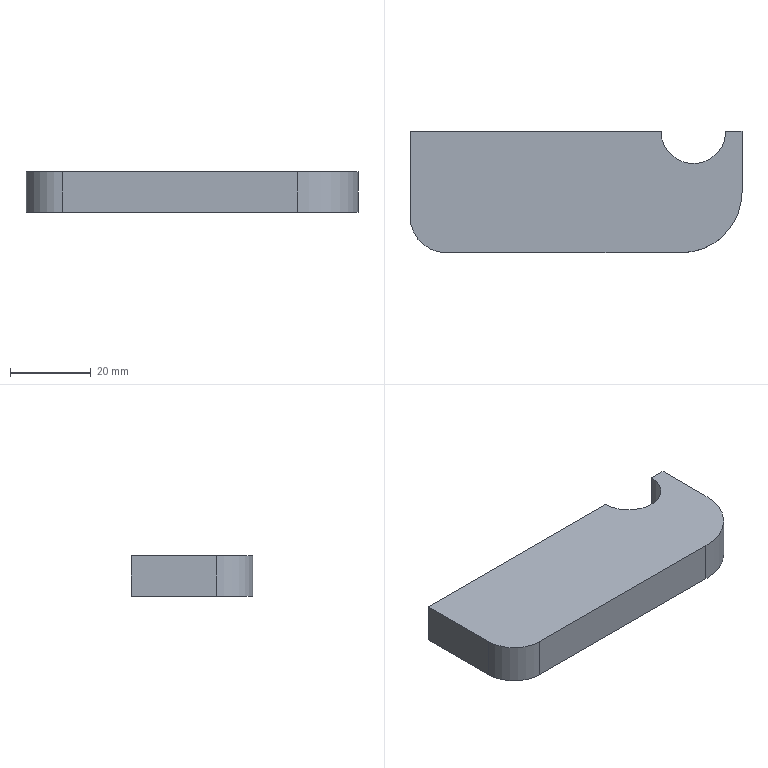Part | STEP file | Part 5_Default<As machined> | 1 solid | 10 faces | box 82 x 30 x 10 mm | volume 22938 mm3 | plane 7 | cylinder 3 | commonest cylinder face diameters 16 x1 18 x1 30 x1
STEP:
#1=CARTESIAN_POINT('',(0.,0.,0.));
#2=DIRECTION('',(0.,0.,1.));
#3=DIRECTION('',(1.,0.,0.));
#4=AXIS2_PLACEMENT_3D('',#1,#2,#3);
#5=CARTESIAN_POINT('',(9.,0.,5.));
#6=VERTEX_POINT('',#5);
#7=CARTESIAN_POINT('',(67.,0.,5.));
#8=VERTEX_POINT('',#7);
#9=CARTESIAN_POINT('',(67.,0.,5.));
#10=DIRECTION('',(1.,0.,0.));
#11=VECTOR('',#10,1.);
#12=LINE('',#9,#11);
#13=CARTESIAN_POINT('',(67.,0.,5.));
#14=DIRECTION('',(0.,1.,0.));
#15=DIRECTION('',(-1.,0.,0.));
#16=AXIS2_PLACEMENT_3D('',#13,#14,#15);
#17=PLANE('',#16);
#18=CARTESIAN_POINT('',(0.,0.));
#19=DIRECTION('',(-1.,0.));
#20=VECTOR('',#19,1.);
#21=LINE('',#18,#20);
#22=(GEOMETRIC_REPRESENTATION_CONTEXT(2)PARAMETRIC_REPRESENTATION_CONTEXT()REPRESENTATION_CONTEXT('',''));
#23=DEFINITIONAL_REPRESENTATION('',(#21),#22);
#24=PCURVE('',#17,#23);
#25=CARTESIAN_POINT('',(70.,30.,5.));
#26=DIRECTION('',(0.,0.,1.));
#27=DIRECTION('',(1.,0.,0.));
#28=AXIS2_PLACEMENT_3D('',#25,#26,#27);
#29=PLANE('',#28);
#30=CARTESIAN_POINT('',(-3.,-30.));
#31=DIRECTION('',(1.,0.));
#32=VECTOR('',#31,1.);
#33=LINE('',#30,#32);
#34=(GEOMETRIC_REPRESENTATION_CONTEXT(2)PARAMETRIC_REPRESENTATION_CONTEXT()REPRESENTATION_CONTEXT('',''));
#35=DEFINITIONAL_REPRESENTATION('',(#33),#34);
#36=PCURVE('',#29,#35);
#37=SURFACE_CURVE('',#12,(#24,#36),.PCURVE_S1.);
#38=EDGE_CURVE('',#6,#8,#37,.T.);
#39=ORIENTED_EDGE('',*,*,#38,.F.);
#40=CARTESIAN_POINT('',(9.,0.,-5.));
#41=VERTEX_POINT('',#40);
#42=CARTESIAN_POINT('',(9.,0.,5.));
#43=DIRECTION('',(0.,0.,-1.));
#44=VECTOR('',#43,1.);
#45=LINE('',#42,#44);
#46=CARTESIAN_POINT('',(58.,0.));
#47=DIRECTION('',(0.,-1.));
#48=VECTOR('',#47,1.);
#49=LINE('',#46,#48);
#50=(GEOMETRIC_REPRESENTATION_CONTEXT(2)PARAMETRIC_REPRESENTATION_CONTEXT()REPRESENTATION_CONTEXT('',''));
#51=DEFINITIONAL_REPRESENTATION('',(#49),#50);
#52=PCURVE('',#17,#51);
#53=CARTESIAN_POINT('',(9.,9.,5.));
#54=DIRECTION('',(0.,0.,-1.));
#55=DIRECTION('',(-1.,0.,0.));
#56=AXIS2_PLACEMENT_3D('',#53,#54,#55);
#57=CYLINDRICAL_SURFACE('',#56,9.);
#58=CARTESIAN_POINT('',(4.712,0.));
#59=DIRECTION('',(0.,1.));
#60=VECTOR('',#59,1.);
#61=LINE('',#58,#60);
#62=(GEOMETRIC_REPRESENTATION_CONTEXT(2)PARAMETRIC_REPRESENTATION_CONTEXT()REPRESENTATION_CONTEXT('',''));
#63=DEFINITIONAL_REPRESENTATION('',(#61),#62);
#64=PCURVE('',#57,#63);
#65=SURFACE_CURVE('',#45,(#52,#64),.PCURVE_S1.);
#66=EDGE_CURVE('',#6,#41,#65,.T.);
#67=ORIENTED_EDGE('',*,*,#66,.T.);
#68=CARTESIAN_POINT('',(67.,0.,-5.));
#69=VERTEX_POINT('',#68);
#70=CARTESIAN_POINT('',(67.,0.,-5.));
#71=DIRECTION('',(1.,0.,0.));
#72=VECTOR('',#71,1.);
#73=LINE('',#70,#72);
#74=CARTESIAN_POINT('',(0.,-10.));
#75=DIRECTION('',(-1.,0.));
#76=VECTOR('',#75,1.);
#77=LINE('',#74,#76);
#78=(GEOMETRIC_REPRESENTATION_CONTEXT(2)PARAMETRIC_REPRESENTATION_CONTEXT()REPRESENTATION_CONTEXT('',''));
#79=DEFINITIONAL_REPRESENTATION('',(#77),#78);
#80=PCURVE('',#17,#79);
#81=CARTESIAN_POINT('',(70.,30.,-5.));
#82=DIRECTION('',(0.,0.,1.));
#83=DIRECTION('',(1.,0.,0.));
#84=AXIS2_PLACEMENT_3D('',#81,#82,#83);
#85=PLANE('',#84);
#86=CARTESIAN_POINT('',(-3.,-30.));
#87=DIRECTION('',(1.,0.));
#88=VECTOR('',#87,1.);
#89=LINE('',#86,#88);
#90=(GEOMETRIC_REPRESENTATION_CONTEXT(2)PARAMETRIC_REPRESENTATION_CONTEXT()REPRESENTATION_CONTEXT('',''));
#91=DEFINITIONAL_REPRESENTATION('',(#89),#90);
#92=PCURVE('',#85,#91);
#93=SURFACE_CURVE('',#73,(#80,#92),.PCURVE_S1.);
#94=EDGE_CURVE('',#41,#69,#93,.T.);
#95=ORIENTED_EDGE('',*,*,#94,.T.);
#96=CARTESIAN_POINT('',(67.,0.,5.));
#97=DIRECTION('',(0.,0.,-1.));
#98=VECTOR('',#97,1.);
#99=LINE('',#96,#98);
#100=CARTESIAN_POINT('',(0.,0.));
#101=DIRECTION('',(0.,-1.));
#102=VECTOR('',#101,1.);
#103=LINE('',#100,#102);
#104=(GEOMETRIC_REPRESENTATION_CONTEXT(2)PARAMETRIC_REPRESENTATION_CONTEXT()REPRESENTATION_CONTEXT('',''));
#105=DEFINITIONAL_REPRESENTATION('',(#103),#104);
#106=PCURVE('',#17,#105);
#107=CARTESIAN_POINT('',(67.,15.,5.));
#108=DIRECTION('',(0.,0.,-1.));
#109=DIRECTION('',(-1.,0.,0.));
#110=AXIS2_PLACEMENT_3D('',#107,#108,#109);
#111=CYLINDRICAL_SURFACE('',#110,15.);
#112=CARTESIAN_POINT('',(4.712,0.));
#113=DIRECTION('',(0.,1.));
#114=VECTOR('',#113,1.);
#115=LINE('',#112,#114);
#116=(GEOMETRIC_REPRESENTATION_CONTEXT(2)PARAMETRIC_REPRESENTATION_CONTEXT()REPRESENTATION_CONTEXT('',''));
#117=DEFINITIONAL_REPRESENTATION('',(#115),#116);
#118=PCURVE('',#111,#117);
#119=SURFACE_CURVE('',#99,(#106,#118),.PCURVE_S1.);
#120=EDGE_CURVE('',#8,#69,#119,.T.);
#121=ORIENTED_EDGE('',*,*,#120,.F.);
#122=EDGE_LOOP('',(#39,#67,#95,#121));
#123=FACE_BOUND('',#122,.T.);
#124=ADVANCED_FACE('',(#123),#17,.F.);
#125=CARTESIAN_POINT('',(82.,15.,-5.));
#126=VERTEX_POINT('',#125);
#127=CARTESIAN_POINT('',(67.,15.,-5.));
#128=DIRECTION('',(0.,0.,1.));
#129=DIRECTION('',(-1.,0.,0.));
#130=AXIS2_PLACEMENT_3D('',#127,#128,#129);
#131=CIRCLE('',#130,15.);
#132=CARTESIAN_POINT('',(6.283,10.));
#133=DIRECTION('',(-1.,0.));
#134=VECTOR('',#133,1.);
#135=LINE('',#132,#134);
#136=(GEOMETRIC_REPRESENTATION_CONTEXT(2)PARAMETRIC_REPRESENTATION_CONTEXT()REPRESENTATION_CONTEXT('',''));
#137=DEFINITIONAL_REPRESENTATION('',(#135),#136);
#138=PCURVE('',#111,#137);
#139=CARTESIAN_POINT('',(-3.,-15.));
#140=DIRECTION('',(-1.,0.));
#141=AXIS2_PLACEMENT_2D('',#139,#140);
#142=CIRCLE('',#141,15.);
#143=(GEOMETRIC_REPRESENTATION_CONTEXT(2)PARAMETRIC_REPRESENTATION_CONTEXT()REPRESENTATION_CONTEXT('',''));
#144=DEFINITIONAL_REPRESENTATION('',(#142),#143);
#145=PCURVE('',#85,#144);
#146=SURFACE_CURVE('',#131,(#138,#145),.PCURVE_S1.);
#147=EDGE_CURVE('',#69,#126,#146,.T.);
#148=ORIENTED_EDGE('',*,*,#147,.T.);
#149=CARTESIAN_POINT('',(82.,15.,5.));
#150=VERTEX_POINT('',#149);
#151=CARTESIAN_POINT('',(82.,15.,5.));
#152=DIRECTION('',(0.,0.,-1.));
#153=VECTOR('',#152,1.);
#154=LINE('',#151,#153);
#155=CARTESIAN_POINT('',(3.142,0.));
#156=DIRECTION('',(0.,1.));
#157=VECTOR('',#156,1.);
#158=LINE('',#155,#157);
#159=(GEOMETRIC_REPRESENTATION_CONTEXT(2)PARAMETRIC_REPRESENTATION_CONTEXT()REPRESENTATION_CONTEXT('',''));
#160=DEFINITIONAL_REPRESENTATION('',(#158),#159);
#161=PCURVE('',#111,#160);
#162=CARTESIAN_POINT('',(82.,30.,5.));
#163=DIRECTION('',(-1.,0.,0.));
#164=DIRECTION('',(0.,-1.,0.));
#165=AXIS2_PLACEMENT_3D('',#162,#163,#164);
#166=PLANE('',#165);
#167=CARTESIAN_POINT('',(15.,0.));
#168=DIRECTION('',(0.,-1.));
#169=VECTOR('',#168,1.);
#170=LINE('',#167,#169);
#171=(GEOMETRIC_REPRESENTATION_CONTEXT(2)PARAMETRIC_REPRESENTATION_CONTEXT()REPRESENTATION_CONTEXT('',''));
#172=DEFINITIONAL_REPRESENTATION('',(#170),#171);
#173=PCURVE('',#166,#172);
#174=SURFACE_CURVE('',#154,(#161,#173),.PCURVE_S1.);
#175=EDGE_CURVE('',#150,#126,#174,.T.);
#176=ORIENTED_EDGE('',*,*,#175,.F.);
#177=CARTESIAN_POINT('',(67.,15.,5.));
#178=DIRECTION('',(0.,0.,1.));
#179=DIRECTION('',(-1.,0.,0.));
#180=AXIS2_PLACEMENT_3D('',#177,#178,#179);
#181=CIRCLE('',#180,15.);
#182=CARTESIAN_POINT('',(6.283,0.));
#183=DIRECTION('',(-1.,0.));
#184=VECTOR('',#183,1.);
#185=LINE('',#182,#184);
#186=(GEOMETRIC_REPRESENTATION_CONTEXT(2)PARAMETRIC_REPRESENTATION_CONTEXT()REPRESENTATION_CONTEXT('',''));
#187=DEFINITIONAL_REPRESENTATION('',(#185),#186);
#188=PCURVE('',#111,#187);
#189=CARTESIAN_POINT('',(-3.,-15.));
#190=DIRECTION('',(-1.,0.));
#191=AXIS2_PLACEMENT_2D('',#189,#190);
#192=CIRCLE('',#191,15.);
#193=(GEOMETRIC_REPRESENTATION_CONTEXT(2)PARAMETRIC_REPRESENTATION_CONTEXT()REPRESENTATION_CONTEXT('',''));
#194=DEFINITIONAL_REPRESENTATION('',(#192),#193);
#195=PCURVE('',#29,#194);
#196=SURFACE_CURVE('',#181,(#188,#195),.PCURVE_S1.);
#197=EDGE_CURVE('',#8,#150,#196,.T.);
#198=ORIENTED_EDGE('',*,*,#197,.F.);
#199=ORIENTED_EDGE('',*,*,#120,.T.);
#200=EDGE_LOOP('',(#148,#176,#198,#199));
#201=FACE_BOUND('',#200,.T.);
#202=ADVANCED_FACE('',(#201),#111,.T.);
#203=CARTESIAN_POINT('',(82.,30.,-5.));
#204=VERTEX_POINT('',#203);
#205=CARTESIAN_POINT('',(82.,30.,-5.));
#206=DIRECTION('',(0.,1.,0.));
#207=VECTOR('',#206,1.);
#208=LINE('',#205,#207);
#209=CARTESIAN_POINT('',(0.,-10.));
#210=DIRECTION('',(-1.,0.));
#211=VECTOR('',#210,1.);
#212=LINE('',#209,#211);
#213=(GEOMETRIC_REPRESENTATION_CONTEXT(2)PARAMETRIC_REPRESENTATION_CONTEXT()REPRESENTATION_CONTEXT('',''));
#214=DEFINITIONAL_REPRESENTATION('',(#212),#213);
#215=PCURVE('',#166,#214);
#216=CARTESIAN_POINT('',(12.,0.));
#217=DIRECTION('',(0.,1.));
#218=VECTOR('',#217,1.);
#219=LINE('',#216,#218);
#220=(GEOMETRIC_REPRESENTATION_CONTEXT(2)PARAMETRIC_REPRESENTATION_CONTEXT()REPRESENTATION_CONTEXT('',''));
#221=DEFINITIONAL_REPRESENTATION('',(#219),#220);
#222=PCURVE('',#85,#221);
#223=SURFACE_CURVE('',#208,(#215,#222),.PCURVE_S1.);
#224=EDGE_CURVE('',#126,#204,#223,.T.);
#225=ORIENTED_EDGE('',*,*,#224,.T.);
#226=CARTESIAN_POINT('',(82.,30.,5.));
#227=VERTEX_POINT('',#226);
#228=CARTESIAN_POINT('',(82.,30.,5.));
#229=DIRECTION('',(0.,0.,-1.));
#230=VECTOR('',#229,1.);
#231=LINE('',#228,#230);
#232=CARTESIAN_POINT('',(0.,0.));
#233=DIRECTION('',(0.,-1.));
#234=VECTOR('',#233,1.);
#235=LINE('',#232,#234);
#236=(GEOMETRIC_REPRESENTATION_CONTEXT(2)PARAMETRIC_REPRESENTATION_CONTEXT()REPRESENTATION_CONTEXT('',''));
#237=DEFINITIONAL_REPRESENTATION('',(#235),#236);
#238=PCURVE('',#166,#237);
#239=CARTESIAN_POINT('',(78.,30.,5.));
#240=DIRECTION('',(0.,-1.,0.));
#241=DIRECTION('',(0.,0.,-1.));
#242=AXIS2_PLACEMENT_3D('',#239,#240,#241);
#243=PLANE('',#242);
#244=CARTESIAN_POINT('',(0.,4.));
#245=DIRECTION('',(1.,0.));
#246=VECTOR('',#245,1.);
#247=LINE('',#244,#246);
#248=(GEOMETRIC_REPRESENTATION_CONTEXT(2)PARAMETRIC_REPRESENTATION_CONTEXT()REPRESENTATION_CONTEXT('',''));
#249=DEFINITIONAL_REPRESENTATION('',(#247),#248);
#250=PCURVE('',#243,#249);
#251=SURFACE_CURVE('',#231,(#238,#250),.PCURVE_S1.);
#252=EDGE_CURVE('',#227,#204,#251,.T.);
#253=ORIENTED_EDGE('',*,*,#252,.F.);
#254=CARTESIAN_POINT('',(82.,30.,5.));
#255=DIRECTION('',(0.,1.,0.));
#256=VECTOR('',#255,1.);
#257=LINE('',#254,#256);
#258=CARTESIAN_POINT('',(0.,0.));
#259=DIRECTION('',(-1.,0.));
#260=VECTOR('',#259,1.);
#261=LINE('',#258,#260);
#262=(GEOMETRIC_REPRESENTATION_CONTEXT(2)PARAMETRIC_REPRESENTATION_CONTEXT()REPRESENTATION_CONTEXT('',''));
#263=DEFINITIONAL_REPRESENTATION('',(#261),#262);
#264=PCURVE('',#166,#263);
#265=CARTESIAN_POINT('',(12.,0.));
#266=DIRECTION('',(0.,1.));
#267=VECTOR('',#266,1.);
#268=LINE('',#265,#267);
#269=(GEOMETRIC_REPRESENTATION_CONTEXT(2)PARAMETRIC_REPRESENTATION_CONTEXT()REPRESENTATION_CONTEXT('',''));
#270=DEFINITIONAL_REPRESENTATION('',(#268),#269);
#271=PCURVE('',#29,#270);
#272=SURFACE_CURVE('',#257,(#264,#271),.PCURVE_S1.);
#273=EDGE_CURVE('',#150,#227,#272,.T.);
#274=ORIENTED_EDGE('',*,*,#273,.F.);
#275=ORIENTED_EDGE('',*,*,#175,.T.);
#276=EDGE_LOOP('',(#225,#253,#274,#275));
#277=FACE_BOUND('',#276,.T.);
#278=ADVANCED_FACE('',(#277),#166,.F.);
#279=CARTESIAN_POINT('',(78.,30.,-5.));
#280=VERTEX_POINT('',#279);
#281=CARTESIAN_POINT('',(78.,30.,-5.));
#282=DIRECTION('',(-1.,0.,0.));
#283=VECTOR('',#282,1.);
#284=LINE('',#281,#283);
#285=CARTESIAN_POINT('',(10.,0.));
#286=DIRECTION('',(0.,-1.));
#287=VECTOR('',#286,1.);
#288=LINE('',#285,#287);
#289=(GEOMETRIC_REPRESENTATION_CONTEXT(2)PARAMETRIC_REPRESENTATION_CONTEXT()REPRESENTATION_CONTEXT('',''));
#290=DEFINITIONAL_REPRESENTATION('',(#288),#289);
#291=PCURVE('',#243,#290);
#292=CARTESIAN_POINT('',(8.,0.));
#293=DIRECTION('',(-1.,0.));
#294=VECTOR('',#293,1.);
#295=LINE('',#292,#294);
#296=(GEOMETRIC_REPRESENTATION_CONTEXT(2)PARAMETRIC_REPRESENTATION_CONTEXT()REPRESENTATION_CONTEXT('',''));
#297=DEFINITIONAL_REPRESENTATION('',(#295),#296);
#298=PCURVE('',#85,#297);
#299=SURFACE_CURVE('',#284,(#291,#298),.PCURVE_S1.);
#300=EDGE_CURVE('',#204,#280,#299,.T.);
#301=ORIENTED_EDGE('',*,*,#300,.T.);
#302=CARTESIAN_POINT('',(78.,30.,5.));
#303=VERTEX_POINT('',#302);
#304=CARTESIAN_POINT('',(78.,30.,5.));
#305=DIRECTION('',(0.,0.,-1.));
#306=VECTOR('',#305,1.);
#307=LINE('',#304,#306);
#308=CARTESIAN_POINT('',(0.,0.));
#309=DIRECTION('',(1.,0.));
#310=VECTOR('',#309,1.);
#311=LINE('',#308,#310);
#312=(GEOMETRIC_REPRESENTATION_CONTEXT(2)PARAMETRIC_REPRESENTATION_CONTEXT()REPRESENTATION_CONTEXT('',''));
#313=DEFINITIONAL_REPRESENTATION('',(#311),#312);
#314=PCURVE('',#243,#313);
#315=CARTESIAN_POINT('',(70.,30.,5.));
#316=DIRECTION('',(0.,0.,-1.));
#317=DIRECTION('',(-1.,0.,0.));
#318=AXIS2_PLACEMENT_3D('',#315,#316,#317);
#319=CYLINDRICAL_SURFACE('',#318,8.);
#320=CARTESIAN_POINT('',(3.142,0.));
#321=DIRECTION('',(0.,1.));
#322=VECTOR('',#321,1.);
#323=LINE('',#320,#322);
#324=(GEOMETRIC_REPRESENTATION_CONTEXT(2)PARAMETRIC_REPRESENTATION_CONTEXT()REPRESENTATION_CONTEXT('',''));
#325=DEFINITIONAL_REPRESENTATION('',(#323),#324);
#326=PCURVE('',#319,#325);
#327=SURFACE_CURVE('',#307,(#314,#326),.PCURVE_S1.);
#328=EDGE_CURVE('',#303,#280,#327,.T.);
#329=ORIENTED_EDGE('',*,*,#328,.F.);
#330=CARTESIAN_POINT('',(78.,30.,5.));
#331=DIRECTION('',(-1.,0.,0.));
#332=VECTOR('',#331,1.);
#333=LINE('',#330,#332);
#334=CARTESIAN_POINT('',(0.,0.));
#335=DIRECTION('',(0.,-1.));
#336=VECTOR('',#335,1.);
#337=LINE('',#334,#336);
#338=(GEOMETRIC_REPRESENTATION_CONTEXT(2)PARAMETRIC_REPRESENTATION_CONTEXT()REPRESENTATION_CONTEXT('',''));
#339=DEFINITIONAL_REPRESENTATION('',(#337),#338);
#340=PCURVE('',#243,#339);
#341=CARTESIAN_POINT('',(8.,0.));
#342=DIRECTION('',(-1.,0.));
#343=VECTOR('',#342,1.);
#344=LINE('',#341,#343);
#345=(GEOMETRIC_REPRESENTATION_CONTEXT(2)PARAMETRIC_REPRESENTATION_CONTEXT()REPRESENTATION_CONTEXT('',''));
#346=DEFINITIONAL_REPRESENTATION('',(#344),#345);
#347=PCURVE('',#29,#346);
#348=SURFACE_CURVE('',#333,(#340,#347),.PCURVE_S1.);
#349=EDGE_CURVE('',#227,#303,#348,.T.);
#350=ORIENTED_EDGE('',*,*,#349,.F.);
#351=ORIENTED_EDGE('',*,*,#252,.T.);
#352=EDGE_LOOP('',(#301,#329,#350,#351));
#353=FACE_BOUND('',#352,.T.);
#354=ADVANCED_FACE('',(#353),#243,.F.);
#355=ORIENTED_EDGE('',*,*,#328,.F.);
#356=CARTESIAN_POINT('',(62.,30.,5.));
#357=VERTEX_POINT('',#356);
#358=CARTESIAN_POINT('',(70.,30.,5.));
#359=DIRECTION('',(0.,0.,-1.));
#360=DIRECTION('',(1.,0.,0.));
#361=AXIS2_PLACEMENT_3D('',#358,#359,#360);
#362=CIRCLE('',#361,8.);
#363=CARTESIAN_POINT('',(3.142,0.));
#364=DIRECTION('',(1.,0.));
#365=VECTOR('',#364,1.);
#366=LINE('',#363,#365);
#367=(GEOMETRIC_REPRESENTATION_CONTEXT(2)PARAMETRIC_REPRESENTATION_CONTEXT()REPRESENTATION_CONTEXT('',''));
#368=DEFINITIONAL_REPRESENTATION('',(#366),#367);
#369=PCURVE('',#319,#368);
#370=CARTESIAN_POINT('',(8.,0.));
#371=CARTESIAN_POINT('',(8.,-13.856));
#372=CARTESIAN_POINT('',(-4.,-6.928));
#373=CARTESIAN_POINT('',(-16.,0.));
#374=CARTESIAN_POINT('',(-4.,6.928));
#375=CARTESIAN_POINT('',(8.,13.856));
#376=CARTESIAN_POINT('',(8.,0.));
#377=(BOUNDED_CURVE()B_SPLINE_CURVE(2,(#370,#371,#372,#373,#374,#375,#376),.UNSPECIFIED.,.T.,.F.)B_SPLINE_CURVE_WITH_KNOTS((1,2,2,2,2,1),(-2.094,0.,2.094,4.189,6.283,8.378),.UNSPECIFIED.)CURVE()GEOMETRIC_REPRESENTATION_ITEM()RATIONAL_B_SPLINE_CURVE((1.,0.5,1.,0.5,1.,0.5,1.))REPRESENTATION_ITEM(''));
#378=(GEOMETRIC_REPRESENTATION_CONTEXT(2)PARAMETRIC_REPRESENTATION_CONTEXT()REPRESENTATION_CONTEXT('',''));
#379=DEFINITIONAL_REPRESENTATION('',(#377),#378);
#380=PCURVE('',#29,#379);
#381=SURFACE_CURVE('',#362,(#369,#380),.PCURVE_S1.);
#382=EDGE_CURVE('',#303,#357,#381,.T.);
#383=ORIENTED_EDGE('',*,*,#382,.T.);
#384=CARTESIAN_POINT('',(62.,30.,-5.));
#385=VERTEX_POINT('',#384);
#386=CARTESIAN_POINT('',(62.,30.,5.));
#387=DIRECTION('',(0.,0.,-1.));
#388=VECTOR('',#387,1.);
#389=LINE('',#386,#388);
#390=CARTESIAN_POINT('',(6.283,0.));
#391=DIRECTION('',(0.,1.));
#392=VECTOR('',#391,1.);
#393=LINE('',#390,#392);
#394=(GEOMETRIC_REPRESENTATION_CONTEXT(2)PARAMETRIC_REPRESENTATION_CONTEXT()REPRESENTATION_CONTEXT('',''));
#395=DEFINITIONAL_REPRESENTATION('',(#393),#394);
#396=PCURVE('',#319,#395);
#397=CARTESIAN_POINT('',(0.,30.,5.));
#398=DIRECTION('',(0.,-1.,0.));
#399=DIRECTION('',(0.,0.,-1.));
#400=AXIS2_PLACEMENT_3D('',#397,#398,#399);
#401=PLANE('',#400);
#402=CARTESIAN_POINT('',(0.,62.));
#403=DIRECTION('',(1.,0.));
#404=VECTOR('',#403,1.);
#405=LINE('',#402,#404);
#406=(GEOMETRIC_REPRESENTATION_CONTEXT(2)PARAMETRIC_REPRESENTATION_CONTEXT()REPRESENTATION_CONTEXT('',''));
#407=DEFINITIONAL_REPRESENTATION('',(#405),#406);
#408=PCURVE('',#401,#407);
#409=SURFACE_CURVE('',#389,(#396,#408),.PCURVE_S1.);
#410=EDGE_CURVE('',#357,#385,#409,.T.);
#411=ORIENTED_EDGE('',*,*,#410,.T.);
#412=CARTESIAN_POINT('',(70.,30.,-5.));
#413=DIRECTION('',(0.,0.,-1.));
#414=DIRECTION('',(1.,0.,0.));
#415=AXIS2_PLACEMENT_3D('',#412,#413,#414);
#416=CIRCLE('',#415,8.);
#417=CARTESIAN_POINT('',(3.142,10.));
#418=DIRECTION('',(1.,0.));
#419=VECTOR('',#418,1.);
#420=LINE('',#417,#419);
#421=(GEOMETRIC_REPRESENTATION_CONTEXT(2)PARAMETRIC_REPRESENTATION_CONTEXT()REPRESENTATION_CONTEXT('',''));
#422=DEFINITIONAL_REPRESENTATION('',(#420),#421);
#423=PCURVE('',#319,#422);
#424=CARTESIAN_POINT('',(8.,0.));
#425=CARTESIAN_POINT('',(8.,-13.856));
#426=CARTESIAN_POINT('',(-4.,-6.928));
#427=CARTESIAN_POINT('',(-16.,0.));
#428=CARTESIAN_POINT('',(-4.,6.928));
#429=CARTESIAN_POINT('',(8.,13.856));
#430=CARTESIAN_POINT('',(8.,0.));
#431=(BOUNDED_CURVE()B_SPLINE_CURVE(2,(#424,#425,#426,#427,#428,#429,#430),.UNSPECIFIED.,.T.,.F.)B_SPLINE_CURVE_WITH_KNOTS((1,2,2,2,2,1),(-2.094,0.,2.094,4.189,6.283,8.378),.UNSPECIFIED.)CURVE()GEOMETRIC_REPRESENTATION_ITEM()RATIONAL_B_SPLINE_CURVE((1.,0.5,1.,0.5,1.,0.5,1.))REPRESENTATION_ITEM(''));
#432=(GEOMETRIC_REPRESENTATION_CONTEXT(2)PARAMETRIC_REPRESENTATION_CONTEXT()REPRESENTATION_CONTEXT('',''));
#433=DEFINITIONAL_REPRESENTATION('',(#431),#432);
#434=PCURVE('',#85,#433);
#435=SURFACE_CURVE('',#416,(#423,#434),.PCURVE_S1.);
#436=EDGE_CURVE('',#280,#385,#435,.T.);
#437=ORIENTED_EDGE('',*,*,#436,.F.);
#438=EDGE_LOOP('',(#355,#383,#411,#437));
#439=FACE_BOUND('',#438,.F.);
#440=ADVANCED_FACE('',(#439),#319,.F.);
#441=CARTESIAN_POINT('',(0.,30.,-5.));
#442=VERTEX_POINT('',#441);
#443=CARTESIAN_POINT('',(0.,30.,-5.));
#444=DIRECTION('',(-1.,0.,0.));
#445=VECTOR('',#444,1.);
#446=LINE('',#443,#445);
#447=CARTESIAN_POINT('',(10.,0.));
#448=DIRECTION('',(0.,-1.));
#449=VECTOR('',#448,1.);
#450=LINE('',#447,#449);
#451=(GEOMETRIC_REPRESENTATION_CONTEXT(2)PARAMETRIC_REPRESENTATION_CONTEXT()REPRESENTATION_CONTEXT('',''));
#452=DEFINITIONAL_REPRESENTATION('',(#450),#451);
#453=PCURVE('',#401,#452);
#454=CARTESIAN_POINT('',(-70.,0.));
#455=DIRECTION('',(-1.,0.));
#456=VECTOR('',#455,1.);
#457=LINE('',#454,#456);
#458=(GEOMETRIC_REPRESENTATION_CONTEXT(2)PARAMETRIC_REPRESENTATION_CONTEXT()REPRESENTATION_CONTEXT('',''));
#459=DEFINITIONAL_REPRESENTATION('',(#457),#458);
#460=PCURVE('',#85,#459);
#461=SURFACE_CURVE('',#446,(#453,#460),.PCURVE_S1.);
#462=EDGE_CURVE('',#385,#442,#461,.T.);
#463=ORIENTED_EDGE('',*,*,#462,.T.);
#464=CARTESIAN_POINT('',(0.,30.,5.));
#465=VERTEX_POINT('',#464);
#466=CARTESIAN_POINT('',(0.,30.,5.));
#467=DIRECTION('',(0.,0.,-1.));
#468=VECTOR('',#467,1.);
#469=LINE('',#466,#468);
#470=CARTESIAN_POINT('',(0.,0.));
#471=DIRECTION('',(1.,0.));
#472=VECTOR('',#471,1.);
#473=LINE('',#470,#472);
#474=(GEOMETRIC_REPRESENTATION_CONTEXT(2)PARAMETRIC_REPRESENTATION_CONTEXT()REPRESENTATION_CONTEXT('',''));
#475=DEFINITIONAL_REPRESENTATION('',(#473),#474);
#476=PCURVE('',#401,#475);
#477=CARTESIAN_POINT('',(0.,0.,5.));
#478=DIRECTION('',(1.,0.,0.));
#479=DIRECTION('',(0.,0.,-1.));
#480=AXIS2_PLACEMENT_3D('',#477,#478,#479);
#481=PLANE('',#480);
#482=CARTESIAN_POINT('',(0.,30.));
#483=DIRECTION('',(1.,0.));
#484=VECTOR('',#483,1.);
#485=LINE('',#482,#484);
#486=(GEOMETRIC_REPRESENTATION_CONTEXT(2)PARAMETRIC_REPRESENTATION_CONTEXT()REPRESENTATION_CONTEXT('',''));
#487=DEFINITIONAL_REPRESENTATION('',(#485),#486);
#488=PCURVE('',#481,#487);
#489=SURFACE_CURVE('',#469,(#476,#488),.PCURVE_S1.);
#490=EDGE_CURVE('',#465,#442,#489,.T.);
#491=ORIENTED_EDGE('',*,*,#490,.F.);
#492=CARTESIAN_POINT('',(0.,30.,5.));
#493=DIRECTION('',(-1.,0.,0.));
#494=VECTOR('',#493,1.);
#495=LINE('',#492,#494);
#496=CARTESIAN_POINT('',(0.,0.));
#497=DIRECTION('',(0.,-1.));
#498=VECTOR('',#497,1.);
#499=LINE('',#496,#498);
#500=(GEOMETRIC_REPRESENTATION_CONTEXT(2)PARAMETRIC_REPRESENTATION_CONTEXT()REPRESENTATION_CONTEXT('',''));
#501=DEFINITIONAL_REPRESENTATION('',(#499),#500);
#502=PCURVE('',#401,#501);
#503=CARTESIAN_POINT('',(-70.,0.));
#504=DIRECTION('',(-1.,0.));
#505=VECTOR('',#504,1.);
#506=LINE('',#503,#505);
#507=(GEOMETRIC_REPRESENTATION_CONTEXT(2)PARAMETRIC_REPRESENTATION_CONTEXT()REPRESENTATION_CONTEXT('',''));
#508=DEFINITIONAL_REPRESENTATION('',(#506),#507);
#509=PCURVE('',#29,#508);
#510=SURFACE_CURVE('',#495,(#502,#509),.PCURVE_S1.);
#511=EDGE_CURVE('',#357,#465,#510,.T.);
#512=ORIENTED_EDGE('',*,*,#511,.F.);
#513=ORIENTED_EDGE('',*,*,#410,.T.);
#514=EDGE_LOOP('',(#463,#491,#512,#513));
#515=FACE_BOUND('',#514,.T.);
#516=ADVANCED_FACE('',(#515),#401,.F.);
#517=CARTESIAN_POINT('',(0.,9.,-5.));
#518=VERTEX_POINT('',#517);
#519=CARTESIAN_POINT('',(0.,0.,-5.));
#520=DIRECTION('',(0.,-1.,0.));
#521=VECTOR('',#520,1.);
#522=LINE('',#519,#521);
#523=CARTESIAN_POINT('',(10.,0.));
#524=DIRECTION('',(0.,-1.));
#525=VECTOR('',#524,1.);
#526=LINE('',#523,#525);
#527=(GEOMETRIC_REPRESENTATION_CONTEXT(2)PARAMETRIC_REPRESENTATION_CONTEXT()REPRESENTATION_CONTEXT('',''));
#528=DEFINITIONAL_REPRESENTATION('',(#526),#527);
#529=PCURVE('',#481,#528);
#530=CARTESIAN_POINT('',(-70.,-30.));
#531=DIRECTION('',(0.,-1.));
#532=VECTOR('',#531,1.);
#533=LINE('',#530,#532);
#534=(GEOMETRIC_REPRESENTATION_CONTEXT(2)PARAMETRIC_REPRESENTATION_CONTEXT()REPRESENTATION_CONTEXT('',''));
#535=DEFINITIONAL_REPRESENTATION('',(#533),#534);
#536=PCURVE('',#85,#535);
#537=SURFACE_CURVE('',#522,(#529,#536),.PCURVE_S1.);
#538=EDGE_CURVE('',#442,#518,#537,.T.);
#539=ORIENTED_EDGE('',*,*,#538,.T.);
#540=CARTESIAN_POINT('',(0.,9.,5.));
#541=VERTEX_POINT('',#540);
#542=CARTESIAN_POINT('',(0.,9.,5.));
#543=DIRECTION('',(0.,0.,1.));
#544=VECTOR('',#543,1.);
#545=LINE('',#542,#544);
#546=CARTESIAN_POINT('',(0.,9.));
#547=DIRECTION('',(-1.,0.));
#548=VECTOR('',#547,1.);
#549=LINE('',#546,#548);
#550=(GEOMETRIC_REPRESENTATION_CONTEXT(2)PARAMETRIC_REPRESENTATION_CONTEXT()REPRESENTATION_CONTEXT('',''));
#551=DEFINITIONAL_REPRESENTATION('',(#549),#550);
#552=PCURVE('',#481,#551);
#553=CARTESIAN_POINT('',(6.283,0.));
#554=DIRECTION('',(0.,-1.));
#555=VECTOR('',#554,1.);
#556=LINE('',#553,#555);
#557=(GEOMETRIC_REPRESENTATION_CONTEXT(2)PARAMETRIC_REPRESENTATION_CONTEXT()REPRESENTATION_CONTEXT('',''));
#558=DEFINITIONAL_REPRESENTATION('',(#556),#557);
#559=PCURVE('',#57,#558);
#560=SURFACE_CURVE('',#545,(#552,#559),.PCURVE_S1.);
#561=EDGE_CURVE('',#518,#541,#560,.T.);
#562=ORIENTED_EDGE('',*,*,#561,.T.);
#563=CARTESIAN_POINT('',(0.,0.,5.));
#564=DIRECTION('',(0.,-1.,0.));
#565=VECTOR('',#564,1.);
#566=LINE('',#563,#565);
#567=CARTESIAN_POINT('',(0.,0.));
#568=DIRECTION('',(0.,-1.));
#569=VECTOR('',#568,1.);
#570=LINE('',#567,#569);
#571=(GEOMETRIC_REPRESENTATION_CONTEXT(2)PARAMETRIC_REPRESENTATION_CONTEXT()REPRESENTATION_CONTEXT('',''));
#572=DEFINITIONAL_REPRESENTATION('',(#570),#571);
#573=PCURVE('',#481,#572);
#574=CARTESIAN_POINT('',(-70.,-30.));
#575=DIRECTION('',(0.,-1.));
#576=VECTOR('',#575,1.);
#577=LINE('',#574,#576);
#578=(GEOMETRIC_REPRESENTATION_CONTEXT(2)PARAMETRIC_REPRESENTATION_CONTEXT()REPRESENTATION_CONTEXT('',''));
#579=DEFINITIONAL_REPRESENTATION('',(#577),#578);
#580=PCURVE('',#29,#579);
#581=SURFACE_CURVE('',#566,(#573,#580),.PCURVE_S1.);
#582=EDGE_CURVE('',#465,#541,#581,.T.);
#583=ORIENTED_EDGE('',*,*,#582,.F.);
#584=ORIENTED_EDGE('',*,*,#490,.T.);
#585=EDGE_LOOP('',(#539,#562,#583,#584));
#586=FACE_BOUND('',#585,.T.);
#587=ADVANCED_FACE('',(#586),#481,.F.);
#588=ORIENTED_EDGE('',*,*,#582,.T.);
#589=CARTESIAN_POINT('',(9.,9.,5.));
#590=DIRECTION('',(0.,0.,1.));
#591=DIRECTION('',(1.,0.,0.));
#592=AXIS2_PLACEMENT_3D('',#589,#590,#591);
#593=CIRCLE('',#592,9.);
#594=CARTESIAN_POINT('',(-61.,-21.));
#595=DIRECTION('',(1.,0.));
#596=AXIS2_PLACEMENT_2D('',#594,#595);
#597=CIRCLE('',#596,9.);
#598=(GEOMETRIC_REPRESENTATION_CONTEXT(2)PARAMETRIC_REPRESENTATION_CONTEXT()REPRESENTATION_CONTEXT('',''));
#599=DEFINITIONAL_REPRESENTATION('',(#597),#598);
#600=PCURVE('',#29,#599);
#601=CARTESIAN_POINT('',(9.425,0.));
#602=DIRECTION('',(-1.,0.));
#603=VECTOR('',#602,1.);
#604=LINE('',#601,#603);
#605=(GEOMETRIC_REPRESENTATION_CONTEXT(2)PARAMETRIC_REPRESENTATION_CONTEXT()REPRESENTATION_CONTEXT('',''));
#606=DEFINITIONAL_REPRESENTATION('',(#604),#605);
#607=PCURVE('',#57,#606);
#608=SURFACE_CURVE('',#593,(#600,#607),.PCURVE_S1.);
#609=EDGE_CURVE('',#541,#6,#608,.T.);
#610=ORIENTED_EDGE('',*,*,#609,.T.);
#611=ORIENTED_EDGE('',*,*,#38,.T.);
#612=ORIENTED_EDGE('',*,*,#197,.T.);
#613=ORIENTED_EDGE('',*,*,#273,.T.);
#614=ORIENTED_EDGE('',*,*,#349,.T.);
#615=ORIENTED_EDGE('',*,*,#382,.T.);
#616=ORIENTED_EDGE('',*,*,#511,.T.);
#617=EDGE_LOOP('',(#588,#610,#611,#612,#613,#614,#615,#616));
#618=FACE_BOUND('',#617,.T.);
#619=ADVANCED_FACE('',(#618),#29,.T.);
#620=ORIENTED_EDGE('',*,*,#94,.F.);
#621=CARTESIAN_POINT('',(9.,9.,-5.));
#622=DIRECTION('',(0.,0.,-1.));
#623=DIRECTION('',(1.,0.,0.));
#624=AXIS2_PLACEMENT_3D('',#621,#622,#623);
#625=CIRCLE('',#624,9.);
#626=CARTESIAN_POINT('',(-52.,-21.));
#627=CARTESIAN_POINT('',(-52.,-36.588));
#628=CARTESIAN_POINT('',(-65.5,-28.794));
#629=CARTESIAN_POINT('',(-79.,-21.));
#630=CARTESIAN_POINT('',(-65.5,-13.206));
#631=CARTESIAN_POINT('',(-52.,-5.412));
#632=CARTESIAN_POINT('',(-52.,-21.));
#633=(BOUNDED_CURVE()B_SPLINE_CURVE(2,(#626,#627,#628,#629,#630,#631,#632),.UNSPECIFIED.,.T.,.F.)B_SPLINE_CURVE_WITH_KNOTS((1,2,2,2,2,1),(-2.094,0.,2.094,4.189,6.283,8.378),.UNSPECIFIED.)CURVE()GEOMETRIC_REPRESENTATION_ITEM()RATIONAL_B_SPLINE_CURVE((1.,0.5,1.,0.5,1.,0.5,1.))REPRESENTATION_ITEM(''));
#634=(GEOMETRIC_REPRESENTATION_CONTEXT(2)PARAMETRIC_REPRESENTATION_CONTEXT()REPRESENTATION_CONTEXT('',''));
#635=DEFINITIONAL_REPRESENTATION('',(#633),#634);
#636=PCURVE('',#85,#635);
#637=CARTESIAN_POINT('',(3.142,10.));
#638=DIRECTION('',(1.,0.));
#639=VECTOR('',#638,1.);
#640=LINE('',#637,#639);
#641=(GEOMETRIC_REPRESENTATION_CONTEXT(2)PARAMETRIC_REPRESENTATION_CONTEXT()REPRESENTATION_CONTEXT('',''));
#642=DEFINITIONAL_REPRESENTATION('',(#640),#641);
#643=PCURVE('',#57,#642);
#644=SURFACE_CURVE('',#625,(#636,#643),.PCURVE_S1.);
#645=EDGE_CURVE('',#41,#518,#644,.T.);
#646=ORIENTED_EDGE('',*,*,#645,.T.);
#647=ORIENTED_EDGE('',*,*,#538,.F.);
#648=ORIENTED_EDGE('',*,*,#462,.F.);
#649=ORIENTED_EDGE('',*,*,#436,.F.);
#650=ORIENTED_EDGE('',*,*,#300,.F.);
#651=ORIENTED_EDGE('',*,*,#224,.F.);
#652=ORIENTED_EDGE('',*,*,#147,.F.);
#653=EDGE_LOOP('',(#620,#646,#647,#648,#649,#650,#651,#652));
#654=FACE_BOUND('',#653,.T.);
#655=ADVANCED_FACE('',(#654),#85,.F.);
#656=ORIENTED_EDGE('',*,*,#609,.F.);
#657=ORIENTED_EDGE('',*,*,#561,.F.);
#658=ORIENTED_EDGE('',*,*,#645,.F.);
#659=ORIENTED_EDGE('',*,*,#66,.F.);
#660=EDGE_LOOP('',(#656,#657,#658,#659));
#661=FACE_BOUND('',#660,.T.);
#662=ADVANCED_FACE('',(#661),#57,.T.);
#663=CLOSED_SHELL('',(#124,#202,#278,#354,#440,#516,#587,#619,#655,#662));
#664=MANIFOLD_SOLID_BREP('',#663);
#665=(LENGTH_UNIT()NAMED_UNIT(*)SI_UNIT(.MILLI.,.METRE.));
#666=UNCERTAINTY_MEASURE_WITH_UNIT(LENGTH_MEASURE(0.0000001),#665,'','');
#667=(NAMED_UNIT(*)PLANE_ANGLE_UNIT()SI_UNIT($,.RADIAN.));
#668=(NAMED_UNIT(*)SI_UNIT($,.STERADIAN.)SOLID_ANGLE_UNIT());
#669=(GEOMETRIC_REPRESENTATION_CONTEXT(3)GLOBAL_UNCERTAINTY_ASSIGNED_CONTEXT((#666))GLOBAL_UNIT_ASSIGNED_CONTEXT((#665,#667,#668))REPRESENTATION_CONTEXT('',''));
#670=ADVANCED_BREP_SHAPE_REPRESENTATION('',(#4,#664),#669);